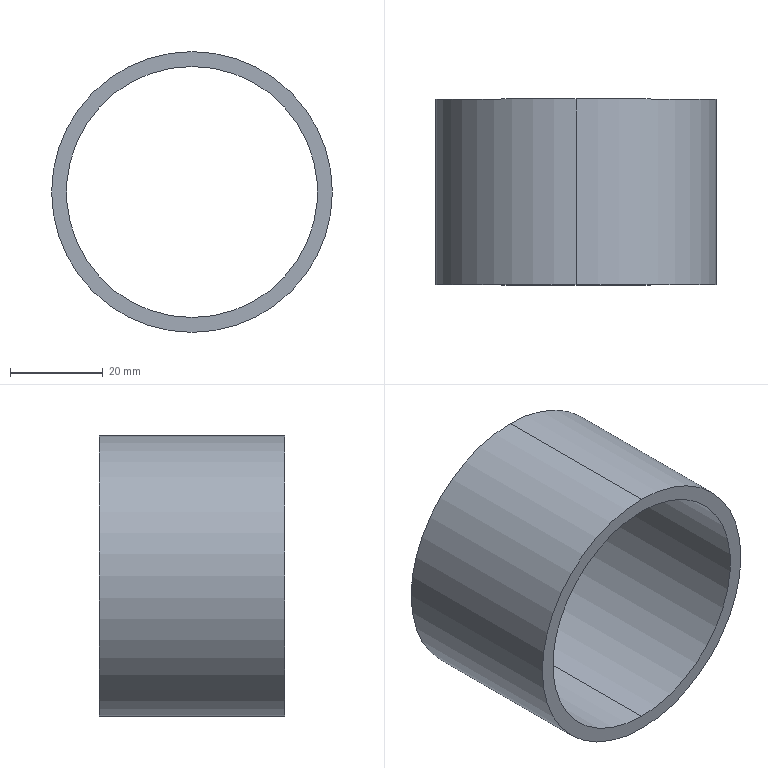Part | SolidWorks | features Extrusion 1 | 1 solid | 6 faces | box 60.5 x 40 x 60.5 mm | volume 23042 mm3 | cylinder 4 | plane 2 | commonest cylinder face diameters 54.1 x2 60.5 x2
STEP:
#1=CARTESIAN_POINT('',(0.,40.,-27.05));
#2=VERTEX_POINT('',#1);
#3=CARTESIAN_POINT('',(0.,40.,27.05));
#4=VERTEX_POINT('',#3);
#5=CARTESIAN_POINT('',(0.,40.,0.));
#6=DIRECTION('',(0.,1.,0.));
#7=DIRECTION('',(0.,0.,1.));
#8=AXIS2_PLACEMENT_3D('',#5,#6,#7);
#9=CIRCLE('',#8,27.05);
#10=EDGE_CURVE('',#2,#4,#9,.T.);
#11=ORIENTED_EDGE('',*,*,#10,.T.);
#12=CARTESIAN_POINT('',(0.,0.,27.05));
#13=VERTEX_POINT('',#12);
#14=CARTESIAN_POINT('',(0.,40.,27.05));
#15=DIRECTION('',(0.,-1.,0.));
#16=VECTOR('',#15,1000.);
#17=LINE('',#14,#16);
#18=EDGE_CURVE('',#4,#13,#17,.T.);
#19=ORIENTED_EDGE('',*,*,#18,.T.);
#20=CARTESIAN_POINT('',(0.,0.,-27.05));
#21=VERTEX_POINT('',#20);
#22=CARTESIAN_POINT('',(0.,0.,0.));
#23=DIRECTION('',(0.,1.,0.));
#24=DIRECTION('',(0.,0.,1.));
#25=AXIS2_PLACEMENT_3D('',#22,#23,#24);
#26=CIRCLE('',#25,27.05);
#27=EDGE_CURVE('',#21,#13,#26,.T.);
#28=ORIENTED_EDGE('',*,*,#27,.F.);
#29=CARTESIAN_POINT('',(0.,40.,-27.05));
#30=DIRECTION('',(0.,-1.,0.));
#31=VECTOR('',#30,1000.);
#32=LINE('',#29,#31);
#33=EDGE_CURVE('',#2,#21,#32,.T.);
#34=ORIENTED_EDGE('',*,*,#33,.F.);
#35=EDGE_LOOP('',(#11,#19,#28,#34));
#36=FACE_OUTER_BOUND('',#35,.T.);
#37=CARTESIAN_POINT('',(0.,40.,0.));
#38=DIRECTION('',(0.,-1.,0.));
#39=DIRECTION('',(0.,0.,-1.));
#40=AXIS2_PLACEMENT_3D('',#37,#38,#39);
#41=CYLINDRICAL_SURFACE('',#40,27.05);
#42=ADVANCED_FACE('',(#36),#41,.F.);
#43=CARTESIAN_POINT('',(0.,40.,30.25));
#44=VERTEX_POINT('',#43);
#45=CARTESIAN_POINT('',(0.,40.,-30.25));
#46=VERTEX_POINT('',#45);
#47=CARTESIAN_POINT('',(0.,40.,0.));
#48=DIRECTION('',(0.,1.,0.));
#49=DIRECTION('',(0.,0.,1.));
#50=AXIS2_PLACEMENT_3D('',#47,#48,#49);
#51=CIRCLE('',#50,30.25);
#52=EDGE_CURVE('',#44,#46,#51,.T.);
#53=ORIENTED_EDGE('',*,*,#52,.F.);
#54=CARTESIAN_POINT('',(0.,0.,30.25));
#55=VERTEX_POINT('',#54);
#56=CARTESIAN_POINT('',(0.,40.,30.25));
#57=DIRECTION('',(0.,-1.,0.));
#58=VECTOR('',#57,1000.);
#59=LINE('',#56,#58);
#60=EDGE_CURVE('',#44,#55,#59,.T.);
#61=ORIENTED_EDGE('',*,*,#60,.T.);
#62=CARTESIAN_POINT('',(0.,0.,-30.25));
#63=VERTEX_POINT('',#62);
#64=CARTESIAN_POINT('',(0.,0.,0.));
#65=DIRECTION('',(0.,1.,0.));
#66=DIRECTION('',(0.,0.,1.));
#67=AXIS2_PLACEMENT_3D('',#64,#65,#66);
#68=CIRCLE('',#67,30.25);
#69=EDGE_CURVE('',#55,#63,#68,.T.);
#70=ORIENTED_EDGE('',*,*,#69,.T.);
#71=CARTESIAN_POINT('',(0.,40.,-30.25));
#72=DIRECTION('',(0.,-1.,0.));
#73=VECTOR('',#72,1000.);
#74=LINE('',#71,#73);
#75=EDGE_CURVE('',#46,#63,#74,.T.);
#76=ORIENTED_EDGE('',*,*,#75,.F.);
#77=EDGE_LOOP('',(#53,#61,#70,#76));
#78=FACE_OUTER_BOUND('',#77,.T.);
#79=CARTESIAN_POINT('',(0.,40.,0.));
#80=DIRECTION('',(0.,-1.,0.));
#81=DIRECTION('',(0.,0.,-1.));
#82=AXIS2_PLACEMENT_3D('',#79,#80,#81);
#83=CYLINDRICAL_SURFACE('',#82,30.25);
#84=ADVANCED_FACE('',(#78),#83,.T.);
#85=CARTESIAN_POINT('',(0.,40.,0.));
#86=DIRECTION('',(0.,1.,0.));
#87=DIRECTION('',(0.,0.,1.));
#88=AXIS2_PLACEMENT_3D('',#85,#86,#87);
#89=CIRCLE('',#88,30.25);
#90=EDGE_CURVE('',#46,#44,#89,.T.);
#91=ORIENTED_EDGE('',*,*,#90,.T.);
#92=ORIENTED_EDGE('',*,*,#52,.T.);
#93=EDGE_LOOP('',(#91,#92));
#94=FACE_OUTER_BOUND('',#93,.T.);
#95=ORIENTED_EDGE('',*,*,#10,.F.);
#96=CARTESIAN_POINT('',(0.,40.,0.));
#97=DIRECTION('',(0.,1.,0.));
#98=DIRECTION('',(0.,0.,1.));
#99=AXIS2_PLACEMENT_3D('',#96,#97,#98);
#100=CIRCLE('',#99,27.05);
#101=EDGE_CURVE('',#4,#2,#100,.T.);
#102=ORIENTED_EDGE('',*,*,#101,.F.);
#103=EDGE_LOOP('',(#95,#102));
#104=FACE_BOUND('',#103,.T.);
#105=CARTESIAN_POINT('',(0.,40.,0.));
#106=DIRECTION('',(0.,1.,0.));
#107=DIRECTION('',(0.,0.,1.));
#108=AXIS2_PLACEMENT_3D('',#105,#106,#107);
#109=PLANE('',#108);
#110=ADVANCED_FACE('',(#94,#104),#109,.T.);
#111=CARTESIAN_POINT('',(0.,0.,0.));
#112=DIRECTION('',(0.,1.,0.));
#113=DIRECTION('',(0.,0.,1.));
#114=AXIS2_PLACEMENT_3D('',#111,#112,#113);
#115=CIRCLE('',#114,30.25);
#116=EDGE_CURVE('',#63,#55,#115,.T.);
#117=ORIENTED_EDGE('',*,*,#116,.F.);
#118=ORIENTED_EDGE('',*,*,#69,.F.);
#119=EDGE_LOOP('',(#117,#118));
#120=FACE_OUTER_BOUND('',#119,.T.);
#121=ORIENTED_EDGE('',*,*,#27,.T.);
#122=CARTESIAN_POINT('',(0.,0.,0.));
#123=DIRECTION('',(0.,1.,0.));
#124=DIRECTION('',(0.,0.,1.));
#125=AXIS2_PLACEMENT_3D('',#122,#123,#124);
#126=CIRCLE('',#125,27.05);
#127=EDGE_CURVE('',#13,#21,#126,.T.);
#128=ORIENTED_EDGE('',*,*,#127,.T.);
#129=EDGE_LOOP('',(#121,#128));
#130=FACE_BOUND('',#129,.T.);
#131=CARTESIAN_POINT('',(0.,0.,0.));
#132=DIRECTION('',(0.,1.,0.));
#133=DIRECTION('',(0.,0.,1.));
#134=AXIS2_PLACEMENT_3D('',#131,#132,#133);
#135=PLANE('',#134);
#136=ADVANCED_FACE('',(#120,#130),#135,.F.);
#137=ORIENTED_EDGE('',*,*,#60,.F.);
#138=ORIENTED_EDGE('',*,*,#90,.F.);
#139=ORIENTED_EDGE('',*,*,#75,.T.);
#140=ORIENTED_EDGE('',*,*,#116,.T.);
#141=EDGE_LOOP('',(#137,#138,#139,#140));
#142=FACE_OUTER_BOUND('',#141,.T.);
#143=CARTESIAN_POINT('',(0.,40.,0.));
#144=DIRECTION('',(0.,-1.,0.));
#145=DIRECTION('',(0.,0.,-1.));
#146=AXIS2_PLACEMENT_3D('',#143,#144,#145);
#147=CYLINDRICAL_SURFACE('',#146,30.25);
#148=ADVANCED_FACE('',(#142),#147,.T.);
#149=ORIENTED_EDGE('',*,*,#18,.F.);
#150=ORIENTED_EDGE('',*,*,#101,.T.);
#151=ORIENTED_EDGE('',*,*,#33,.T.);
#152=ORIENTED_EDGE('',*,*,#127,.F.);
#153=EDGE_LOOP('',(#149,#150,#151,#152));
#154=FACE_OUTER_BOUND('',#153,.T.);
#155=CARTESIAN_POINT('',(0.,40.,0.));
#156=DIRECTION('',(0.,-1.,0.));
#157=DIRECTION('',(0.,0.,-1.));
#158=AXIS2_PLACEMENT_3D('',#155,#156,#157);
#159=CYLINDRICAL_SURFACE('',#158,27.05);
#160=ADVANCED_FACE('',(#154),#159,.F.);
#161=CLOSED_SHELL('',(#42,#84,#110,#136,#148,#160));
#162=MANIFOLD_SOLID_BREP('',#161);
#163=CARTESIAN_POINT('',(0.,0.,0.));
#164=DIRECTION('',(0.,0.,1.));
#165=DIRECTION('',(1.,0.,0.));
#166=AXIS2_PLACEMENT_3D('',#163,#164,#165);
#167=(LENGTH_UNIT()NAMED_UNIT(*)SI_UNIT(.MILLI.,.METRE.));
#168=UNCERTAINTY_MEASURE_WITH_UNIT(LENGTH_MEASURE(0.00001),#167,'','');
#169=(NAMED_UNIT(*)PLANE_ANGLE_UNIT()SI_UNIT($,.RADIAN.));
#170=(NAMED_UNIT(*)SI_UNIT($,.STERADIAN.)SOLID_ANGLE_UNIT());
#171=(GEOMETRIC_REPRESENTATION_CONTEXT(3)GLOBAL_UNCERTAINTY_ASSIGNED_CONTEXT((#168))GLOBAL_UNIT_ASSIGNED_CONTEXT((#167,#169,#170))REPRESENTATION_CONTEXT('',''));
#172=ADVANCED_BREP_SHAPE_REPRESENTATION('',(#162,#166),#171);